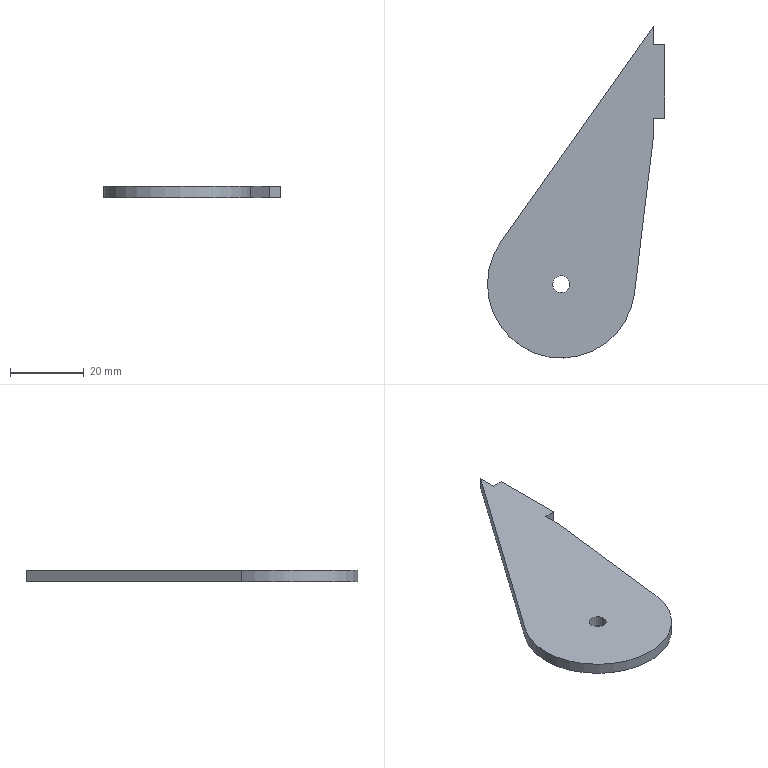Part | SolidWorks | features ICE 2, Extrusion 1 | 1 solid | 12 faces | box 48 x 90 x 3 mm | volume 6866 mm3 | plane 9 | cylinder 3 | commonest cylinder face diameters 4.6 x2 40 x1
STEP:
#1=CARTESIAN_POINT('',(-2.3,0.,-3.));
#2=VERTEX_POINT('',#1);
#3=CARTESIAN_POINT('',(2.3,0.,-3.));
#4=VERTEX_POINT('',#3);
#5=CARTESIAN_POINT('',(0.,0.,-3.));
#6=DIRECTION('',(0.,0.,1.));
#7=DIRECTION('',(1.,0.,0.));
#8=AXIS2_PLACEMENT_3D('',#5,#6,#7);
#9=CIRCLE('',#8,2.3);
#10=EDGE_CURVE('',#2,#4,#9,.T.);
#11=ORIENTED_EDGE('',*,*,#10,.F.);
#12=CARTESIAN_POINT('',(-2.3,0.,0.));
#13=VERTEX_POINT('',#12);
#14=CARTESIAN_POINT('',(-2.3,0.,-10.));
#15=DIRECTION('',(0.,0.,1.));
#16=VECTOR('',#15,1000.);
#17=LINE('',#14,#16);
#18=EDGE_CURVE('',#2,#13,#17,.T.);
#19=ORIENTED_EDGE('',*,*,#18,.T.);
#20=CARTESIAN_POINT('',(2.3,0.,0.));
#21=VERTEX_POINT('',#20);
#22=CARTESIAN_POINT('',(0.,0.,0.));
#23=DIRECTION('',(0.,0.,1.));
#24=DIRECTION('',(1.,0.,0.));
#25=AXIS2_PLACEMENT_3D('',#22,#23,#24);
#26=CIRCLE('',#25,2.3);
#27=EDGE_CURVE('',#13,#21,#26,.T.);
#28=ORIENTED_EDGE('',*,*,#27,.T.);
#29=CARTESIAN_POINT('',(2.3,0.,-10.));
#30=DIRECTION('',(0.,0.,1.));
#31=VECTOR('',#30,1000.);
#32=LINE('',#29,#31);
#33=EDGE_CURVE('',#4,#21,#32,.T.);
#34=ORIENTED_EDGE('',*,*,#33,.F.);
#35=EDGE_LOOP('',(#11,#19,#28,#34));
#36=FACE_OUTER_BOUND('',#35,.T.);
#37=CARTESIAN_POINT('',(0.,0.,-10.));
#38=DIRECTION('',(0.,0.,1.));
#39=DIRECTION('',(1.,0.,0.));
#40=AXIS2_PLACEMENT_3D('',#37,#38,#39);
#41=CYLINDRICAL_SURFACE('',#40,2.3);
#42=ADVANCED_FACE('',(#36),#41,.F.);
#43=CARTESIAN_POINT('',(25.,65.,-3.));
#44=VERTEX_POINT('',#43);
#45=CARTESIAN_POINT('',(25.,65.,0.));
#46=VERTEX_POINT('',#45);
#47=CARTESIAN_POINT('',(25.,65.,0.));
#48=DIRECTION('',(0.,0.,1.));
#49=VECTOR('',#48,1000.);
#50=LINE('',#47,#49);
#51=EDGE_CURVE('',#44,#46,#50,.T.);
#52=ORIENTED_EDGE('',*,*,#51,.F.);
#53=CARTESIAN_POINT('',(25.,70.,-3.));
#54=VERTEX_POINT('',#53);
#55=CARTESIAN_POINT('',(25.,70.,-3.));
#56=DIRECTION('',(0.,1.,0.));
#57=VECTOR('',#56,1000.);
#58=LINE('',#55,#57);
#59=EDGE_CURVE('',#44,#54,#58,.T.);
#60=ORIENTED_EDGE('',*,*,#59,.T.);
#61=CARTESIAN_POINT('',(25.,70.,0.));
#62=VERTEX_POINT('',#61);
#63=CARTESIAN_POINT('',(25.,70.,-3.));
#64=DIRECTION('',(0.,0.,1.));
#65=VECTOR('',#64,1000.);
#66=LINE('',#63,#65);
#67=EDGE_CURVE('',#54,#62,#66,.T.);
#68=ORIENTED_EDGE('',*,*,#67,.T.);
#69=CARTESIAN_POINT('',(25.,70.,0.));
#70=DIRECTION('',(0.,1.,0.));
#71=VECTOR('',#70,1000.);
#72=LINE('',#69,#71);
#73=EDGE_CURVE('',#46,#62,#72,.T.);
#74=ORIENTED_EDGE('',*,*,#73,.F.);
#75=EDGE_LOOP('',(#52,#60,#68,#74));
#76=FACE_OUTER_BOUND('',#75,.T.);
#77=CARTESIAN_POINT('',(25.,70.,-3.));
#78=DIRECTION('',(1.,0.,0.));
#79=DIRECTION('',(0.,1.,0.));
#80=AXIS2_PLACEMENT_3D('',#77,#78,#79);
#81=PLANE('',#80);
#82=ADVANCED_FACE('',(#76),#81,.T.);
#83=CARTESIAN_POINT('',(-16.33,11.547,0.));
#84=VERTEX_POINT('',#83);
#85=CARTESIAN_POINT('',(19.854,-2.409,0.));
#86=VERTEX_POINT('',#85);
#87=CARTESIAN_POINT('',(0.,0.,0.));
#88=DIRECTION('',(0.,0.,1.));
#89=DIRECTION('',(1.,0.,0.));
#90=AXIS2_PLACEMENT_3D('',#87,#88,#89);
#91=CIRCLE('',#90,20.);
#92=EDGE_CURVE('',#84,#86,#91,.T.);
#93=ORIENTED_EDGE('',*,*,#92,.F.);
#94=CARTESIAN_POINT('',(-16.33,11.547,-3.));
#95=VERTEX_POINT('',#94);
#96=CARTESIAN_POINT('',(-16.33,11.547,-3.));
#97=DIRECTION('',(0.,0.,1.));
#98=VECTOR('',#97,1000.);
#99=LINE('',#96,#98);
#100=EDGE_CURVE('',#95,#84,#99,.T.);
#101=ORIENTED_EDGE('',*,*,#100,.F.);
#102=CARTESIAN_POINT('',(19.854,-2.409,-3.));
#103=VERTEX_POINT('',#102);
#104=CARTESIAN_POINT('',(0.,0.,-3.));
#105=DIRECTION('',(0.,0.,1.));
#106=DIRECTION('',(1.,0.,0.));
#107=AXIS2_PLACEMENT_3D('',#104,#105,#106);
#108=CIRCLE('',#107,20.);
#109=EDGE_CURVE('',#95,#103,#108,.T.);
#110=ORIENTED_EDGE('',*,*,#109,.T.);
#111=CARTESIAN_POINT('',(19.854,-2.409,-3.));
#112=DIRECTION('',(0.,0.,1.));
#113=VECTOR('',#112,1000.);
#114=LINE('',#111,#113);
#115=EDGE_CURVE('',#103,#86,#114,.T.);
#116=ORIENTED_EDGE('',*,*,#115,.T.);
#117=EDGE_LOOP('',(#93,#101,#110,#116));
#118=FACE_OUTER_BOUND('',#117,.T.);
#119=CARTESIAN_POINT('',(0.,0.,-3.));
#120=DIRECTION('',(0.,0.,1.));
#121=DIRECTION('',(1.,0.,0.));
#122=AXIS2_PLACEMENT_3D('',#119,#120,#121);
#123=CYLINDRICAL_SURFACE('',#122,20.);
#124=ADVANCED_FACE('',(#118),#123,.T.);
#125=CARTESIAN_POINT('',(-16.33,11.547,0.));
#126=DIRECTION('',(-0.5773,-0.8165,0.));
#127=VECTOR('',#126,1000.);
#128=LINE('',#125,#127);
#129=EDGE_CURVE('',#62,#84,#128,.T.);
#130=ORIENTED_EDGE('',*,*,#129,.F.);
#131=ORIENTED_EDGE('',*,*,#67,.F.);
#132=CARTESIAN_POINT('',(-16.33,11.547,-3.));
#133=DIRECTION('',(-0.5773,-0.8165,0.));
#134=VECTOR('',#133,1000.);
#135=LINE('',#132,#134);
#136=EDGE_CURVE('',#54,#95,#135,.T.);
#137=ORIENTED_EDGE('',*,*,#136,.T.);
#138=ORIENTED_EDGE('',*,*,#100,.T.);
#139=EDGE_LOOP('',(#130,#131,#137,#138));
#140=FACE_OUTER_BOUND('',#139,.T.);
#141=CARTESIAN_POINT('',(-16.33,11.547,-3.));
#142=DIRECTION('',(-0.8165,0.5773,0.));
#143=DIRECTION('',(-0.5773,-0.8165,0.));
#144=AXIS2_PLACEMENT_3D('',#141,#142,#143);
#145=PLANE('',#144);
#146=ADVANCED_FACE('',(#140),#145,.T.);
#147=CARTESIAN_POINT('',(25.,45.,0.));
#148=VERTEX_POINT('',#147);
#149=CARTESIAN_POINT('',(25.,45.,-3.));
#150=VERTEX_POINT('',#149);
#151=CARTESIAN_POINT('',(25.,45.,0.));
#152=DIRECTION('',(0.,0.,-1.));
#153=VECTOR('',#152,1000.);
#154=LINE('',#151,#153);
#155=EDGE_CURVE('',#148,#150,#154,.T.);
#156=ORIENTED_EDGE('',*,*,#155,.F.);
#157=CARTESIAN_POINT('',(25.,40.,0.));
#158=VERTEX_POINT('',#157);
#159=CARTESIAN_POINT('',(25.,70.,0.));
#160=DIRECTION('',(0.,1.,0.));
#161=VECTOR('',#160,1000.);
#162=LINE('',#159,#161);
#163=EDGE_CURVE('',#158,#148,#162,.T.);
#164=ORIENTED_EDGE('',*,*,#163,.F.);
#165=CARTESIAN_POINT('',(25.,40.,-3.));
#166=VERTEX_POINT('',#165);
#167=CARTESIAN_POINT('',(25.,40.,-3.));
#168=DIRECTION('',(0.,0.,1.));
#169=VECTOR('',#168,1000.);
#170=LINE('',#167,#169);
#171=EDGE_CURVE('',#166,#158,#170,.T.);
#172=ORIENTED_EDGE('',*,*,#171,.F.);
#173=CARTESIAN_POINT('',(25.,70.,-3.));
#174=DIRECTION('',(0.,1.,0.));
#175=VECTOR('',#174,1000.);
#176=LINE('',#173,#175);
#177=EDGE_CURVE('',#166,#150,#176,.T.);
#178=ORIENTED_EDGE('',*,*,#177,.T.);
#179=EDGE_LOOP('',(#156,#164,#172,#178));
#180=FACE_OUTER_BOUND('',#179,.T.);
#181=CARTESIAN_POINT('',(25.,70.,-3.));
#182=DIRECTION('',(1.,0.,0.));
#183=DIRECTION('',(0.,1.,0.));
#184=AXIS2_PLACEMENT_3D('',#181,#182,#183);
#185=PLANE('',#184);
#186=ADVANCED_FACE('',(#180),#185,.T.);
#187=CARTESIAN_POINT('',(25.,40.,0.));
#188=DIRECTION('',(0.1204,0.9927,0.));
#189=VECTOR('',#188,1000.);
#190=LINE('',#187,#189);
#191=EDGE_CURVE('',#86,#158,#190,.T.);
#192=ORIENTED_EDGE('',*,*,#191,.F.);
#193=ORIENTED_EDGE('',*,*,#115,.F.);
#194=CARTESIAN_POINT('',(25.,40.,-3.));
#195=DIRECTION('',(0.1204,0.9927,0.));
#196=VECTOR('',#195,1000.);
#197=LINE('',#194,#196);
#198=EDGE_CURVE('',#103,#166,#197,.T.);
#199=ORIENTED_EDGE('',*,*,#198,.T.);
#200=ORIENTED_EDGE('',*,*,#171,.T.);
#201=EDGE_LOOP('',(#192,#193,#199,#200));
#202=FACE_OUTER_BOUND('',#201,.T.);
#203=CARTESIAN_POINT('',(25.,40.,-3.));
#204=DIRECTION('',(0.9927,-0.1204,0.));
#205=DIRECTION('',(0.1204,0.9927,0.));
#206=AXIS2_PLACEMENT_3D('',#203,#204,#205);
#207=PLANE('',#206);
#208=ADVANCED_FACE('',(#202),#207,.T.);
#209=CARTESIAN_POINT('',(0.,0.,-3.));
#210=DIRECTION('',(0.,0.,1.));
#211=DIRECTION('',(1.,0.,0.));
#212=AXIS2_PLACEMENT_3D('',#209,#210,#211);
#213=CIRCLE('',#212,2.3);
#214=EDGE_CURVE('',#4,#2,#213,.T.);
#215=ORIENTED_EDGE('',*,*,#214,.T.);
#216=ORIENTED_EDGE('',*,*,#10,.T.);
#217=EDGE_LOOP('',(#215,#216));
#218=FACE_BOUND('',#217,.T.);
#219=ORIENTED_EDGE('',*,*,#109,.F.);
#220=ORIENTED_EDGE('',*,*,#136,.F.);
#221=ORIENTED_EDGE('',*,*,#59,.F.);
#222=CARTESIAN_POINT('',(28.,65.,-3.));
#223=VERTEX_POINT('',#222);
#224=CARTESIAN_POINT('',(28.,65.,-3.));
#225=DIRECTION('',(-1.,0.,0.));
#226=VECTOR('',#225,1000.);
#227=LINE('',#224,#226);
#228=EDGE_CURVE('',#223,#44,#227,.T.);
#229=ORIENTED_EDGE('',*,*,#228,.F.);
#230=CARTESIAN_POINT('',(28.,45.,-3.));
#231=VERTEX_POINT('',#230);
#232=CARTESIAN_POINT('',(28.,65.,-3.));
#233=DIRECTION('',(0.,1.,0.));
#234=VECTOR('',#233,1000.);
#235=LINE('',#232,#234);
#236=EDGE_CURVE('',#231,#223,#235,.T.);
#237=ORIENTED_EDGE('',*,*,#236,.F.);
#238=CARTESIAN_POINT('',(28.,45.,-3.));
#239=DIRECTION('',(-1.,0.,0.));
#240=VECTOR('',#239,1000.);
#241=LINE('',#238,#240);
#242=EDGE_CURVE('',#231,#150,#241,.T.);
#243=ORIENTED_EDGE('',*,*,#242,.T.);
#244=ORIENTED_EDGE('',*,*,#177,.F.);
#245=ORIENTED_EDGE('',*,*,#198,.F.);
#246=EDGE_LOOP('',(#219,#220,#221,#229,#237,#243,#244,#245));
#247=FACE_OUTER_BOUND('',#246,.T.);
#248=CARTESIAN_POINT('',(0.,0.,-3.));
#249=DIRECTION('',(0.,0.,1.));
#250=DIRECTION('',(1.,0.,0.));
#251=AXIS2_PLACEMENT_3D('',#248,#249,#250);
#252=PLANE('',#251);
#253=ADVANCED_FACE('',(#218,#247),#252,.F.);
#254=CARTESIAN_POINT('',(0.,0.,0.));
#255=DIRECTION('',(0.,0.,1.));
#256=DIRECTION('',(1.,0.,0.));
#257=AXIS2_PLACEMENT_3D('',#254,#255,#256);
#258=CIRCLE('',#257,2.3);
#259=EDGE_CURVE('',#21,#13,#258,.T.);
#260=ORIENTED_EDGE('',*,*,#259,.F.);
#261=ORIENTED_EDGE('',*,*,#27,.F.);
#262=EDGE_LOOP('',(#260,#261));
#263=FACE_BOUND('',#262,.T.);
#264=ORIENTED_EDGE('',*,*,#92,.T.);
#265=ORIENTED_EDGE('',*,*,#191,.T.);
#266=ORIENTED_EDGE('',*,*,#163,.T.);
#267=CARTESIAN_POINT('',(28.,45.,0.));
#268=VERTEX_POINT('',#267);
#269=CARTESIAN_POINT('',(28.,45.,0.));
#270=DIRECTION('',(-1.,0.,0.));
#271=VECTOR('',#270,1000.);
#272=LINE('',#269,#271);
#273=EDGE_CURVE('',#268,#148,#272,.T.);
#274=ORIENTED_EDGE('',*,*,#273,.F.);
#275=CARTESIAN_POINT('',(28.,65.,0.));
#276=VERTEX_POINT('',#275);
#277=CARTESIAN_POINT('',(28.,65.,0.));
#278=DIRECTION('',(0.,-1.,0.));
#279=VECTOR('',#278,1000.);
#280=LINE('',#277,#279);
#281=EDGE_CURVE('',#276,#268,#280,.T.);
#282=ORIENTED_EDGE('',*,*,#281,.F.);
#283=CARTESIAN_POINT('',(28.,65.,0.));
#284=DIRECTION('',(-1.,0.,0.));
#285=VECTOR('',#284,1000.);
#286=LINE('',#283,#285);
#287=EDGE_CURVE('',#276,#46,#286,.T.);
#288=ORIENTED_EDGE('',*,*,#287,.T.);
#289=ORIENTED_EDGE('',*,*,#73,.T.);
#290=ORIENTED_EDGE('',*,*,#129,.T.);
#291=EDGE_LOOP('',(#264,#265,#266,#274,#282,#288,#289,#290));
#292=FACE_OUTER_BOUND('',#291,.T.);
#293=CARTESIAN_POINT('',(0.,0.,0.));
#294=DIRECTION('',(0.,0.,1.));
#295=DIRECTION('',(1.,0.,0.));
#296=AXIS2_PLACEMENT_3D('',#293,#294,#295);
#297=PLANE('',#296);
#298=ADVANCED_FACE('',(#263,#292),#297,.T.);
#299=ORIENTED_EDGE('',*,*,#18,.F.);
#300=ORIENTED_EDGE('',*,*,#214,.F.);
#301=ORIENTED_EDGE('',*,*,#33,.T.);
#302=ORIENTED_EDGE('',*,*,#259,.T.);
#303=EDGE_LOOP('',(#299,#300,#301,#302));
#304=FACE_OUTER_BOUND('',#303,.T.);
#305=CARTESIAN_POINT('',(0.,0.,-10.));
#306=DIRECTION('',(0.,0.,1.));
#307=DIRECTION('',(1.,0.,0.));
#308=AXIS2_PLACEMENT_3D('',#305,#306,#307);
#309=CYLINDRICAL_SURFACE('',#308,2.3);
#310=ADVANCED_FACE('',(#304),#309,.F.);
#311=ORIENTED_EDGE('',*,*,#155,.T.);
#312=ORIENTED_EDGE('',*,*,#242,.F.);
#313=CARTESIAN_POINT('',(28.,45.,0.));
#314=DIRECTION('',(0.,0.,-1.));
#315=VECTOR('',#314,1000.);
#316=LINE('',#313,#315);
#317=EDGE_CURVE('',#268,#231,#316,.T.);
#318=ORIENTED_EDGE('',*,*,#317,.F.);
#319=ORIENTED_EDGE('',*,*,#273,.T.);
#320=EDGE_LOOP('',(#311,#312,#318,#319));
#321=FACE_OUTER_BOUND('',#320,.T.);
#322=CARTESIAN_POINT('',(28.,45.,0.));
#323=DIRECTION('',(0.,1.,0.));
#324=DIRECTION('',(-1.,0.,0.));
#325=AXIS2_PLACEMENT_3D('',#322,#323,#324);
#326=PLANE('',#325);
#327=ADVANCED_FACE('',(#321),#326,.F.);
#328=ORIENTED_EDGE('',*,*,#51,.T.);
#329=ORIENTED_EDGE('',*,*,#287,.F.);
#330=CARTESIAN_POINT('',(28.,65.,0.));
#331=DIRECTION('',(0.,0.,1.));
#332=VECTOR('',#331,1000.);
#333=LINE('',#330,#332);
#334=EDGE_CURVE('',#223,#276,#333,.T.);
#335=ORIENTED_EDGE('',*,*,#334,.F.);
#336=ORIENTED_EDGE('',*,*,#228,.T.);
#337=EDGE_LOOP('',(#328,#329,#335,#336));
#338=FACE_OUTER_BOUND('',#337,.T.);
#339=CARTESIAN_POINT('',(28.,65.,0.));
#340=DIRECTION('',(0.,-1.,0.));
#341=DIRECTION('',(1.,0.,0.));
#342=AXIS2_PLACEMENT_3D('',#339,#340,#341);
#343=PLANE('',#342);
#344=ADVANCED_FACE('',(#338),#343,.F.);
#345=ORIENTED_EDGE('',*,*,#281,.T.);
#346=ORIENTED_EDGE('',*,*,#317,.T.);
#347=ORIENTED_EDGE('',*,*,#236,.T.);
#348=ORIENTED_EDGE('',*,*,#334,.T.);
#349=EDGE_LOOP('',(#345,#346,#347,#348));
#350=FACE_OUTER_BOUND('',#349,.T.);
#351=CARTESIAN_POINT('',(28.,0.,0.));
#352=DIRECTION('',(1.,0.,0.));
#353=DIRECTION('',(0.,1.,0.));
#354=AXIS2_PLACEMENT_3D('',#351,#352,#353);
#355=PLANE('',#354);
#356=ADVANCED_FACE('',(#350),#355,.T.);
#357=CLOSED_SHELL('',(#42,#82,#124,#146,#186,#208,#253,#298,#310,#327,#344,#356));
#358=MANIFOLD_SOLID_BREP('',#357);
#359=CARTESIAN_POINT('',(0.,0.,0.));
#360=DIRECTION('',(0.,0.,1.));
#361=DIRECTION('',(1.,0.,0.));
#362=AXIS2_PLACEMENT_3D('',#359,#360,#361);
#363=(LENGTH_UNIT()NAMED_UNIT(*)SI_UNIT(.MILLI.,.METRE.));
#364=UNCERTAINTY_MEASURE_WITH_UNIT(LENGTH_MEASURE(0.00001),#363,'','');
#365=(NAMED_UNIT(*)PLANE_ANGLE_UNIT()SI_UNIT($,.RADIAN.));
#366=(NAMED_UNIT(*)SI_UNIT($,.STERADIAN.)SOLID_ANGLE_UNIT());
#367=(GEOMETRIC_REPRESENTATION_CONTEXT(3)GLOBAL_UNCERTAINTY_ASSIGNED_CONTEXT((#364))GLOBAL_UNIT_ASSIGNED_CONTEXT((#363,#365,#366))REPRESENTATION_CONTEXT('',''));
#368=ADVANCED_BREP_SHAPE_REPRESENTATION('',(#358,#362),#367);